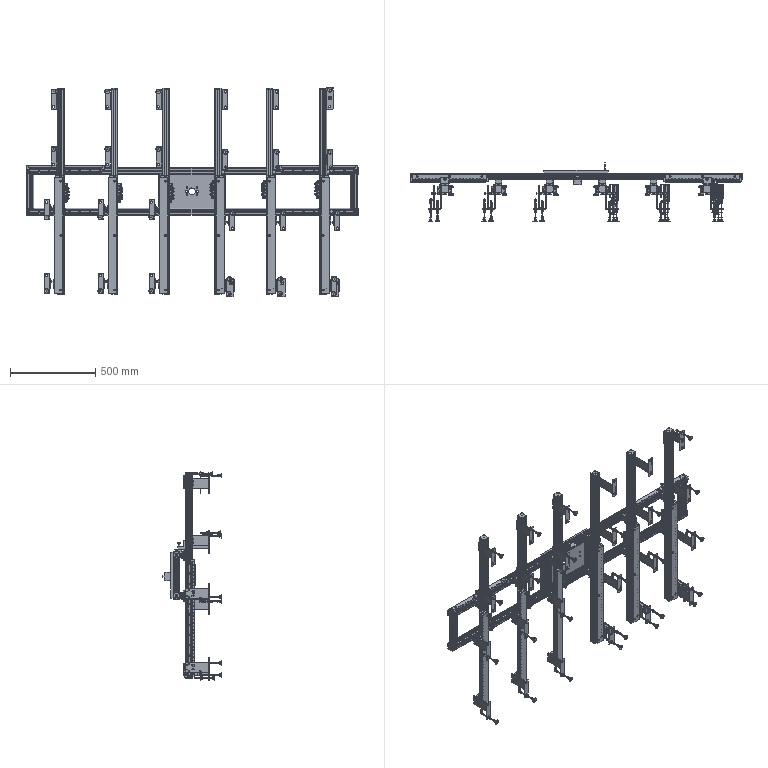Part | SolidWorks | features ReferencePattern 15, CompositeCurve 4, MirrorCompFeat 4, LocalLPattern 1 | 297 solids | 23334 faces | volume 15004104 mm3 | plane 10177 | cylinder 7264 | cone 4003 | spline 1890 | commonest cylinder face diameters 4.1 x480 4 x406 7 x363 6 x352 10 x338 8 x328